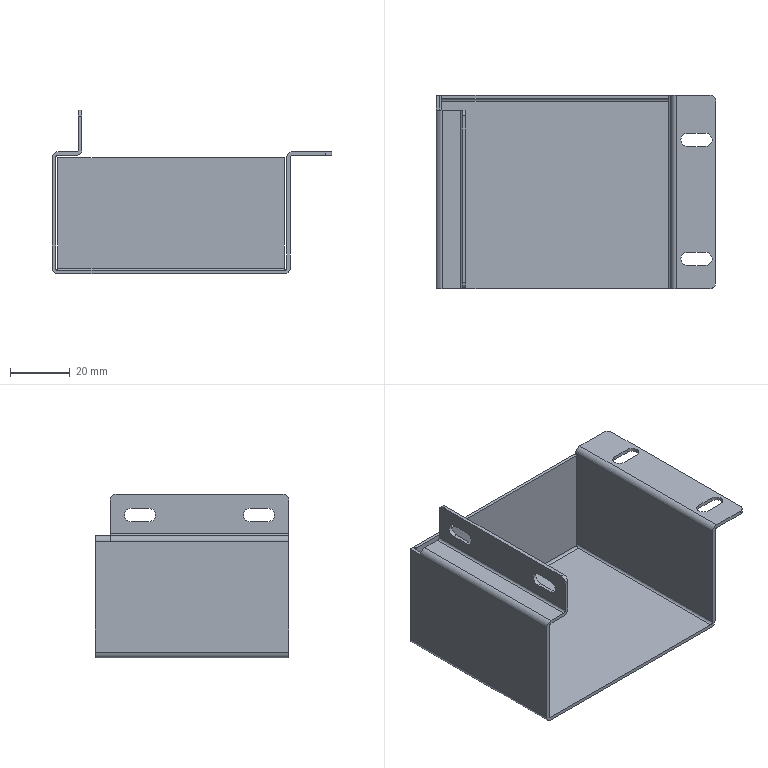Part | SolidWorks | features BaseBody 1 | 1 solid | 60 faces | box 94 x 65 x 55 mm | volume 18142 mm3 | plane 34 | cylinder 26 | commonest cylinder face diameters 4.5 x10 1.473 x5 3.873 x5 4 x5 1.6 x1